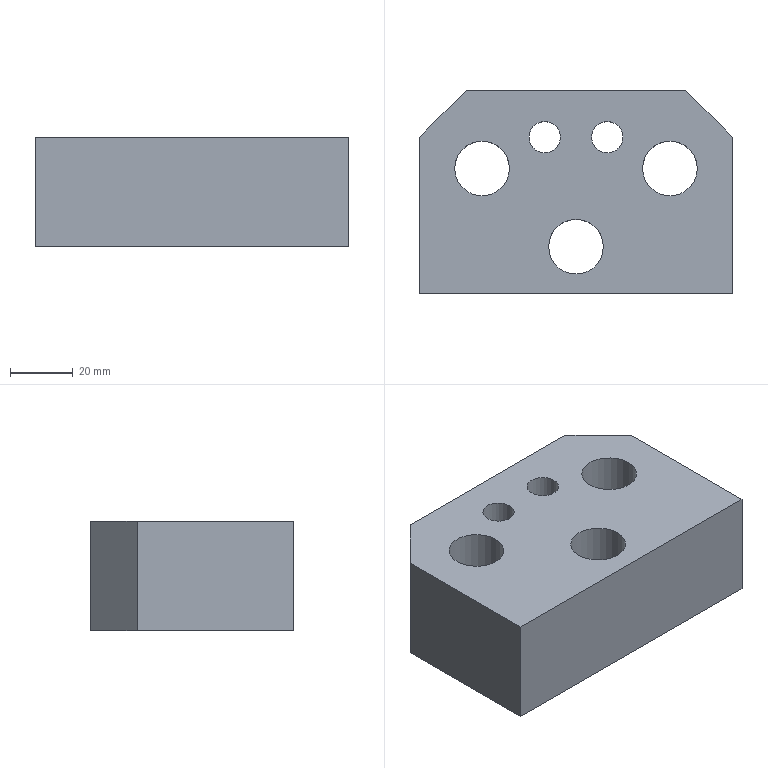Part | NX | features solid 2 | 1 solid | 17 faces | box 100 x 65 x 35 mm | volume 188377 mm3 | plane 10 | cylinder 7 | commonest cylinder face diameters 17.5 x3 10 x2 11 x2
STEP:
#1=CARTESIAN_POINT('',(392.5,-135.,35.));
#2=VERTEX_POINT('',#1);
#3=CARTESIAN_POINT('',(387.5,-135.,35.));
#4=DIRECTION('',(0.,0.,1.));
#5=DIRECTION('',(1.,0.,0.));
#6=AXIS2_PLACEMENT_3D('',#3,#4,#5);
#7=CIRCLE('',#6,5.);
#8=EDGE_CURVE('',#2,#2,#7,.T.);
#9=ORIENTED_EDGE('',*,*,#8,.F.);
#10=EDGE_LOOP('',(#9));
#11=FACE_BOUND('',#10,.T.);
#12=CARTESIAN_POINT('',(412.5,-135.,35.));
#13=VERTEX_POINT('',#12);
#14=CARTESIAN_POINT('',(407.5,-135.,35.));
#15=DIRECTION('',(0.,0.,1.));
#16=DIRECTION('',(1.,0.,0.));
#17=AXIS2_PLACEMENT_3D('',#14,#15,#16);
#18=CIRCLE('',#17,5.);
#19=EDGE_CURVE('',#13,#13,#18,.T.);
#20=ORIENTED_EDGE('',*,*,#19,.F.);
#21=EDGE_LOOP('',(#20));
#22=FACE_BOUND('',#21,.T.);
#23=CARTESIAN_POINT('',(447.5,-185.,35.));
#24=VERTEX_POINT('',#23);
#25=CARTESIAN_POINT('',(347.5,-185.,35.));
#26=VERTEX_POINT('',#25);
#27=CARTESIAN_POINT('',(372.5,-185.,35.));
#28=DIRECTION('',(-1.,0.,0.));
#29=VECTOR('',#28,1000.);
#30=LINE('',#27,#29);
#31=EDGE_CURVE('',#24,#26,#30,.T.);
#32=ORIENTED_EDGE('',*,*,#31,.F.);
#33=CARTESIAN_POINT('',(447.5,-135.,35.));
#34=VERTEX_POINT('',#33);
#35=CARTESIAN_POINT('',(447.5,-190.,35.));
#36=DIRECTION('',(0.,1.,0.));
#37=VECTOR('',#36,1000.);
#38=LINE('',#35,#37);
#39=EDGE_CURVE('',#24,#34,#38,.T.);
#40=ORIENTED_EDGE('',*,*,#39,.T.);
#41=CARTESIAN_POINT('',(432.5,-120.,35.));
#42=VERTEX_POINT('',#41);
#43=CARTESIAN_POINT('',(432.5,-120.,35.));
#44=DIRECTION('',(0.7071,-0.7071,0.));
#45=VECTOR('',#44,1000.);
#46=LINE('',#43,#45);
#47=EDGE_CURVE('',#34,#42,#46,.F.);
#48=ORIENTED_EDGE('',*,*,#47,.T.);
#49=CARTESIAN_POINT('',(362.5,-120.,35.));
#50=VERTEX_POINT('',#49);
#51=CARTESIAN_POINT('',(447.5,-120.,35.));
#52=DIRECTION('',(1.,0.,0.));
#53=VECTOR('',#52,1000.);
#54=LINE('',#51,#53);
#55=EDGE_CURVE('',#50,#42,#54,.T.);
#56=ORIENTED_EDGE('',*,*,#55,.F.);
#57=CARTESIAN_POINT('',(347.5,-135.,35.));
#58=VERTEX_POINT('',#57);
#59=CARTESIAN_POINT('',(337.5,-145.,35.));
#60=DIRECTION('',(0.7071,0.7071,0.));
#61=VECTOR('',#60,1000.);
#62=LINE('',#59,#61);
#63=EDGE_CURVE('',#50,#58,#62,.F.);
#64=ORIENTED_EDGE('',*,*,#63,.T.);
#65=CARTESIAN_POINT('',(347.5,-190.,35.));
#66=DIRECTION('',(0.,1.,0.));
#67=VECTOR('',#66,1000.);
#68=LINE('',#65,#67);
#69=EDGE_CURVE('',#26,#58,#68,.T.);
#70=ORIENTED_EDGE('',*,*,#69,.F.);
#71=EDGE_LOOP('',(#32,#40,#48,#56,#64,#70));
#72=FACE_BOUND('',#71,.T.);
#73=CARTESIAN_POINT('',(376.25,-145.,35.));
#74=VERTEX_POINT('',#73);
#75=CARTESIAN_POINT('',(367.5,-145.,35.));
#76=DIRECTION('',(0.,0.,1.));
#77=DIRECTION('',(1.,0.,0.));
#78=AXIS2_PLACEMENT_3D('',#75,#76,#77);
#79=CIRCLE('',#78,8.75);
#80=EDGE_CURVE('',#74,#74,#79,.T.);
#81=ORIENTED_EDGE('',*,*,#80,.F.);
#82=EDGE_LOOP('',(#81));
#83=FACE_BOUND('',#82,.T.);
#84=CARTESIAN_POINT('',(436.25,-145.,35.));
#85=VERTEX_POINT('',#84);
#86=CARTESIAN_POINT('',(427.5,-145.,35.));
#87=DIRECTION('',(0.,0.,1.));
#88=DIRECTION('',(1.,0.,0.));
#89=AXIS2_PLACEMENT_3D('',#86,#87,#88);
#90=CIRCLE('',#89,8.75);
#91=EDGE_CURVE('',#85,#85,#90,.T.);
#92=ORIENTED_EDGE('',*,*,#91,.F.);
#93=EDGE_LOOP('',(#92));
#94=FACE_BOUND('',#93,.T.);
#95=CARTESIAN_POINT('',(406.25,-170.,35.));
#96=VERTEX_POINT('',#95);
#97=CARTESIAN_POINT('',(397.5,-170.,35.));
#98=DIRECTION('',(0.,0.,1.));
#99=DIRECTION('',(1.,0.,0.));
#100=AXIS2_PLACEMENT_3D('',#97,#98,#99);
#101=CIRCLE('',#100,8.75);
#102=EDGE_CURVE('',#96,#96,#101,.T.);
#103=ORIENTED_EDGE('',*,*,#102,.F.);
#104=EDGE_LOOP('',(#103));
#105=FACE_BOUND('',#104,.T.);
#106=CARTESIAN_POINT('',(372.5,-190.,35.));
#107=DIRECTION('',(0.,0.,1.));
#108=DIRECTION('',(1.,0.,0.));
#109=AXIS2_PLACEMENT_3D('',#106,#107,#108);
#110=PLANE('',#109);
#111=ADVANCED_FACE('',(#11,#22,#72,#83,#94,#105),#110,.T.);
#112=CARTESIAN_POINT('',(447.5,-185.,0.));
#113=VERTEX_POINT('',#112);
#114=CARTESIAN_POINT('',(447.5,-185.,100.));
#115=DIRECTION('',(0.,0.,-1.));
#116=VECTOR('',#115,1000.);
#117=LINE('',#114,#116);
#118=EDGE_CURVE('',#24,#113,#117,.T.);
#119=ORIENTED_EDGE('',*,*,#118,.T.);
#120=CARTESIAN_POINT('',(447.5,-135.,0.));
#121=VERTEX_POINT('',#120);
#122=CARTESIAN_POINT('',(447.5,-190.,0.));
#123=DIRECTION('',(0.,1.,0.));
#124=VECTOR('',#123,1000.);
#125=LINE('',#122,#124);
#126=EDGE_CURVE('',#113,#121,#125,.T.);
#127=ORIENTED_EDGE('',*,*,#126,.T.);
#128=CARTESIAN_POINT('',(447.5,-135.,25.));
#129=DIRECTION('',(0.,0.,1.));
#130=VECTOR('',#129,1000.);
#131=LINE('',#128,#130);
#132=EDGE_CURVE('',#121,#34,#131,.T.);
#133=ORIENTED_EDGE('',*,*,#132,.T.);
#134=ORIENTED_EDGE('',*,*,#39,.F.);
#135=EDGE_LOOP('',(#119,#127,#133,#134));
#136=FACE_BOUND('',#135,.T.);
#137=CARTESIAN_POINT('',(447.5,-190.,25.));
#138=DIRECTION('',(1.,0.,0.));
#139=DIRECTION('',(0.,0.,-1.));
#140=AXIS2_PLACEMENT_3D('',#137,#138,#139);
#141=PLANE('',#140);
#142=ADVANCED_FACE('',(#136),#141,.T.);
#143=CARTESIAN_POINT('',(382.,-135.,0.));
#144=VERTEX_POINT('',#143);
#145=CARTESIAN_POINT('',(387.5,-135.,0.));
#146=DIRECTION('',(0.,0.,-1.));
#147=DIRECTION('',(-1.,0.,0.));
#148=AXIS2_PLACEMENT_3D('',#145,#146,#147);
#149=CIRCLE('',#148,5.5);
#150=EDGE_CURVE('',#144,#144,#149,.T.);
#151=ORIENTED_EDGE('',*,*,#150,.F.);
#152=EDGE_LOOP('',(#151));
#153=FACE_BOUND('',#152,.T.);
#154=CARTESIAN_POINT('',(402.,-135.,0.));
#155=VERTEX_POINT('',#154);
#156=CARTESIAN_POINT('',(407.5,-135.,0.));
#157=DIRECTION('',(0.,0.,-1.));
#158=DIRECTION('',(-1.,0.,0.));
#159=AXIS2_PLACEMENT_3D('',#156,#157,#158);
#160=CIRCLE('',#159,5.5);
#161=EDGE_CURVE('',#155,#155,#160,.T.);
#162=ORIENTED_EDGE('',*,*,#161,.F.);
#163=EDGE_LOOP('',(#162));
#164=FACE_BOUND('',#163,.T.);
#165=CARTESIAN_POINT('',(347.5,-185.,0.));
#166=VERTEX_POINT('',#165);
#167=CARTESIAN_POINT('',(447.5,-185.,0.));
#168=DIRECTION('',(-1.,0.,0.));
#169=VECTOR('',#168,1000.);
#170=LINE('',#167,#169);
#171=EDGE_CURVE('',#113,#166,#170,.T.);
#172=ORIENTED_EDGE('',*,*,#171,.T.);
#173=CARTESIAN_POINT('',(347.5,-135.,0.));
#174=VERTEX_POINT('',#173);
#175=CARTESIAN_POINT('',(347.5,-190.,0.));
#176=DIRECTION('',(0.,1.,0.));
#177=VECTOR('',#176,1000.);
#178=LINE('',#175,#177);
#179=EDGE_CURVE('',#166,#174,#178,.T.);
#180=ORIENTED_EDGE('',*,*,#179,.T.);
#181=CARTESIAN_POINT('',(362.5,-120.,0.));
#182=VERTEX_POINT('',#181);
#183=CARTESIAN_POINT('',(332.5,-150.,0.));
#184=DIRECTION('',(-0.7071,-0.7071,0.));
#185=VECTOR('',#184,1000.);
#186=LINE('',#183,#185);
#187=EDGE_CURVE('',#174,#182,#186,.F.);
#188=ORIENTED_EDGE('',*,*,#187,.T.);
#189=CARTESIAN_POINT('',(432.5,-120.,0.));
#190=VERTEX_POINT('',#189);
#191=CARTESIAN_POINT('',(447.5,-120.,0.));
#192=DIRECTION('',(-1.,0.,0.));
#193=VECTOR('',#192,1000.);
#194=LINE('',#191,#193);
#195=EDGE_CURVE('',#190,#182,#194,.T.);
#196=ORIENTED_EDGE('',*,*,#195,.F.);
#197=CARTESIAN_POINT('',(437.5,-125.,0.));
#198=DIRECTION('',(-0.7071,0.7071,0.));
#199=VECTOR('',#198,1000.);
#200=LINE('',#197,#199);
#201=EDGE_CURVE('',#190,#121,#200,.F.);
#202=ORIENTED_EDGE('',*,*,#201,.T.);
#203=ORIENTED_EDGE('',*,*,#126,.F.);
#204=EDGE_LOOP('',(#172,#180,#188,#196,#202,#203));
#205=FACE_BOUND('',#204,.T.);
#206=CARTESIAN_POINT('',(376.25,-145.,0.));
#207=VERTEX_POINT('',#206);
#208=CARTESIAN_POINT('',(367.5,-145.,0.));
#209=DIRECTION('',(0.,0.,1.));
#210=DIRECTION('',(1.,0.,0.));
#211=AXIS2_PLACEMENT_3D('',#208,#209,#210);
#212=CIRCLE('',#211,8.75);
#213=EDGE_CURVE('',#207,#207,#212,.T.);
#214=ORIENTED_EDGE('',*,*,#213,.T.);
#215=EDGE_LOOP('',(#214));
#216=FACE_BOUND('',#215,.T.);
#217=CARTESIAN_POINT('',(436.25,-145.,0.));
#218=VERTEX_POINT('',#217);
#219=CARTESIAN_POINT('',(427.5,-145.,0.));
#220=DIRECTION('',(0.,0.,1.));
#221=DIRECTION('',(1.,0.,0.));
#222=AXIS2_PLACEMENT_3D('',#219,#220,#221);
#223=CIRCLE('',#222,8.75);
#224=EDGE_CURVE('',#218,#218,#223,.T.);
#225=ORIENTED_EDGE('',*,*,#224,.T.);
#226=EDGE_LOOP('',(#225));
#227=FACE_BOUND('',#226,.T.);
#228=CARTESIAN_POINT('',(406.25,-170.,0.));
#229=VERTEX_POINT('',#228);
#230=CARTESIAN_POINT('',(397.5,-170.,0.));
#231=DIRECTION('',(0.,0.,1.));
#232=DIRECTION('',(1.,0.,0.));
#233=AXIS2_PLACEMENT_3D('',#230,#231,#232);
#234=CIRCLE('',#233,8.75);
#235=EDGE_CURVE('',#229,#229,#234,.T.);
#236=ORIENTED_EDGE('',*,*,#235,.T.);
#237=EDGE_LOOP('',(#236));
#238=FACE_BOUND('',#237,.T.);
#239=CARTESIAN_POINT('',(372.5,-190.,0.));
#240=DIRECTION('',(0.,0.,-1.));
#241=DIRECTION('',(-1.,0.,0.));
#242=AXIS2_PLACEMENT_3D('',#239,#240,#241);
#243=PLANE('',#242);
#244=ADVANCED_FACE('',(#153,#164,#205,#216,#227,#238),#243,.T.);
#245=CARTESIAN_POINT('',(347.5,-185.,0.));
#246=DIRECTION('',(0.,0.,1.));
#247=VECTOR('',#246,1000.);
#248=LINE('',#245,#247);
#249=EDGE_CURVE('',#166,#26,#248,.T.);
#250=ORIENTED_EDGE('',*,*,#249,.T.);
#251=ORIENTED_EDGE('',*,*,#69,.T.);
#252=CARTESIAN_POINT('',(347.5,-135.,-75.));
#253=DIRECTION('',(0.,0.,-1.));
#254=VECTOR('',#253,1000.);
#255=LINE('',#252,#254);
#256=EDGE_CURVE('',#58,#174,#255,.T.);
#257=ORIENTED_EDGE('',*,*,#256,.T.);
#258=ORIENTED_EDGE('',*,*,#179,.F.);
#259=EDGE_LOOP('',(#250,#251,#257,#258));
#260=FACE_BOUND('',#259,.T.);
#261=CARTESIAN_POINT('',(347.5,-190.,-75.));
#262=DIRECTION('',(-1.,0.,0.));
#263=DIRECTION('',(0.,0.,1.));
#264=AXIS2_PLACEMENT_3D('',#261,#262,#263);
#265=PLANE('',#264);
#266=ADVANCED_FACE('',(#260),#265,.T.);
#267=ORIENTED_EDGE('',*,*,#55,.T.);
#268=CARTESIAN_POINT('',(432.5,-120.,25.));
#269=DIRECTION('',(0.,0.,-1.));
#270=VECTOR('',#269,1000.);
#271=LINE('',#268,#270);
#272=EDGE_CURVE('',#42,#190,#271,.T.);
#273=ORIENTED_EDGE('',*,*,#272,.T.);
#274=ORIENTED_EDGE('',*,*,#195,.T.);
#275=CARTESIAN_POINT('',(362.5,-120.,25.));
#276=DIRECTION('',(0.,0.,1.));
#277=VECTOR('',#276,1000.);
#278=LINE('',#275,#277);
#279=EDGE_CURVE('',#182,#50,#278,.T.);
#280=ORIENTED_EDGE('',*,*,#279,.T.);
#281=EDGE_LOOP('',(#267,#273,#274,#280));
#282=FACE_BOUND('',#281,.T.);
#283=CARTESIAN_POINT('',(447.5,-120.,25.));
#284=DIRECTION('',(0.,1.,0.));
#285=DIRECTION('',(-1.,0.,0.));
#286=AXIS2_PLACEMENT_3D('',#283,#284,#285);
#287=PLANE('',#286);
#288=ADVANCED_FACE('',(#282),#287,.T.);
#289=ORIENTED_EDGE('',*,*,#47,.F.);
#290=ORIENTED_EDGE('',*,*,#132,.F.);
#291=ORIENTED_EDGE('',*,*,#201,.F.);
#292=ORIENTED_EDGE('',*,*,#272,.F.);
#293=EDGE_LOOP('',(#289,#290,#291,#292));
#294=FACE_BOUND('',#293,.T.);
#295=CARTESIAN_POINT('',(432.5,-120.,25.));
#296=DIRECTION('',(-0.7071,-0.7071,0.));
#297=DIRECTION('',(0.7071,-0.7071,0.));
#298=AXIS2_PLACEMENT_3D('',#295,#296,#297);
#299=PLANE('',#298);
#300=ADVANCED_FACE('',(#294),#299,.F.);
#301=ORIENTED_EDGE('',*,*,#187,.F.);
#302=ORIENTED_EDGE('',*,*,#256,.F.);
#303=ORIENTED_EDGE('',*,*,#63,.F.);
#304=ORIENTED_EDGE('',*,*,#279,.F.);
#305=EDGE_LOOP('',(#301,#302,#303,#304));
#306=FACE_BOUND('',#305,.T.);
#307=CARTESIAN_POINT('',(362.5,-120.,25.));
#308=DIRECTION('',(0.7071,-0.7071,0.));
#309=DIRECTION('',(0.7071,0.7071,0.));
#310=AXIS2_PLACEMENT_3D('',#307,#308,#309);
#311=PLANE('',#310);
#312=ADVANCED_FACE('',(#306),#311,.F.);
#313=ORIENTED_EDGE('',*,*,#102,.T.);
#314=EDGE_LOOP('',(#313));
#315=FACE_BOUND('',#314,.T.);
#316=ORIENTED_EDGE('',*,*,#235,.F.);
#317=EDGE_LOOP('',(#316));
#318=FACE_BOUND('',#317,.T.);
#319=CARTESIAN_POINT('',(397.5,-170.,125.));
#320=DIRECTION('',(0.,0.,1.));
#321=DIRECTION('',(1.,0.,0.));
#322=AXIS2_PLACEMENT_3D('',#319,#320,#321);
#323=CYLINDRICAL_SURFACE('',#322,8.75);
#324=ADVANCED_FACE('',(#315,#318),#323,.F.);
#325=ORIENTED_EDGE('',*,*,#91,.T.);
#326=EDGE_LOOP('',(#325));
#327=FACE_BOUND('',#326,.T.);
#328=ORIENTED_EDGE('',*,*,#224,.F.);
#329=EDGE_LOOP('',(#328));
#330=FACE_BOUND('',#329,.T.);
#331=CARTESIAN_POINT('',(427.5,-145.,125.));
#332=DIRECTION('',(0.,0.,1.));
#333=DIRECTION('',(1.,0.,0.));
#334=AXIS2_PLACEMENT_3D('',#331,#332,#333);
#335=CYLINDRICAL_SURFACE('',#334,8.75);
#336=ADVANCED_FACE('',(#327,#330),#335,.F.);
#337=ORIENTED_EDGE('',*,*,#80,.T.);
#338=EDGE_LOOP('',(#337));
#339=FACE_BOUND('',#338,.T.);
#340=ORIENTED_EDGE('',*,*,#213,.F.);
#341=EDGE_LOOP('',(#340));
#342=FACE_BOUND('',#341,.T.);
#343=CARTESIAN_POINT('',(367.5,-145.,125.));
#344=DIRECTION('',(0.,0.,1.));
#345=DIRECTION('',(1.,0.,0.));
#346=AXIS2_PLACEMENT_3D('',#343,#344,#345);
#347=CYLINDRICAL_SURFACE('',#346,8.75);
#348=ADVANCED_FACE('',(#339,#342),#347,.F.);
#349=ORIENTED_EDGE('',*,*,#31,.T.);
#350=ORIENTED_EDGE('',*,*,#249,.F.);
#351=ORIENTED_EDGE('',*,*,#171,.F.);
#352=ORIENTED_EDGE('',*,*,#118,.F.);
#353=EDGE_LOOP('',(#349,#350,#351,#352));
#354=FACE_BOUND('',#353,.T.);
#355=CARTESIAN_POINT('',(447.5,-185.,100.));
#356=DIRECTION('',(0.,1.,0.));
#357=DIRECTION('',(-1.,0.,0.));
#358=AXIS2_PLACEMENT_3D('',#355,#356,#357);
#359=PLANE('',#358);
#360=ADVANCED_FACE('',(#354),#359,.F.);
#361=ORIENTED_EDGE('',*,*,#19,.T.);
#362=EDGE_LOOP('',(#361));
#363=FACE_BOUND('',#362,.T.);
#364=CARTESIAN_POINT('',(412.5,-135.,15.));
#365=VERTEX_POINT('',#364);
#366=CARTESIAN_POINT('',(407.5,-135.,15.));
#367=DIRECTION('',(0.,0.,1.));
#368=DIRECTION('',(1.,0.,0.));
#369=AXIS2_PLACEMENT_3D('',#366,#367,#368);
#370=CIRCLE('',#369,5.);
#371=EDGE_CURVE('',#365,#365,#370,.F.);
#372=ORIENTED_EDGE('',*,*,#371,.T.);
#373=EDGE_LOOP('',(#372));
#374=FACE_BOUND('',#373,.T.);
#375=CARTESIAN_POINT('',(407.5,-135.,55.));
#376=DIRECTION('',(0.,0.,-1.));
#377=DIRECTION('',(-1.,0.,0.));
#378=AXIS2_PLACEMENT_3D('',#375,#376,#377);
#379=CYLINDRICAL_SURFACE('',#378,5.);
#380=ADVANCED_FACE('',(#363,#374),#379,.F.);
#381=ORIENTED_EDGE('',*,*,#371,.F.);
#382=EDGE_LOOP('',(#381));
#383=FACE_BOUND('',#382,.T.);
#384=CARTESIAN_POINT('',(402.,-135.,15.));
#385=VERTEX_POINT('',#384);
#386=CARTESIAN_POINT('',(407.5,-135.,15.));
#387=DIRECTION('',(0.,0.,-1.));
#388=DIRECTION('',(-1.,0.,0.));
#389=AXIS2_PLACEMENT_3D('',#386,#387,#388);
#390=CIRCLE('',#389,5.5);
#391=EDGE_CURVE('',#385,#385,#390,.T.);
#392=ORIENTED_EDGE('',*,*,#391,.T.);
#393=EDGE_LOOP('',(#392));
#394=FACE_BOUND('',#393,.T.);
#395=CARTESIAN_POINT('',(404.011,-134.928,15.));
#396=DIRECTION('',(0.,0.,1.));
#397=DIRECTION('',(1.,0.,0.));
#398=AXIS2_PLACEMENT_3D('',#395,#396,#397);
#399=PLANE('',#398);
#400=ADVANCED_FACE('',(#383,#394),#399,.F.);
#401=ORIENTED_EDGE('',*,*,#161,.T.);
#402=EDGE_LOOP('',(#401));
#403=FACE_BOUND('',#402,.T.);
#404=ORIENTED_EDGE('',*,*,#391,.F.);
#405=EDGE_LOOP('',(#404));
#406=FACE_BOUND('',#405,.T.);
#407=CARTESIAN_POINT('',(407.5,-135.,15.));
#408=DIRECTION('',(0.,0.,-1.));
#409=DIRECTION('',(-1.,0.,0.));
#410=AXIS2_PLACEMENT_3D('',#407,#408,#409);
#411=CYLINDRICAL_SURFACE('',#410,5.5);
#412=ADVANCED_FACE('',(#403,#406),#411,.F.);
#413=ORIENTED_EDGE('',*,*,#8,.T.);
#414=EDGE_LOOP('',(#413));
#415=FACE_BOUND('',#414,.T.);
#416=CARTESIAN_POINT('',(392.5,-135.,15.));
#417=VERTEX_POINT('',#416);
#418=CARTESIAN_POINT('',(387.5,-135.,15.));
#419=DIRECTION('',(0.,0.,1.));
#420=DIRECTION('',(1.,0.,0.));
#421=AXIS2_PLACEMENT_3D('',#418,#419,#420);
#422=CIRCLE('',#421,5.);
#423=EDGE_CURVE('',#417,#417,#422,.F.);
#424=ORIENTED_EDGE('',*,*,#423,.T.);
#425=EDGE_LOOP('',(#424));
#426=FACE_BOUND('',#425,.T.);
#427=CARTESIAN_POINT('',(387.5,-135.,55.));
#428=DIRECTION('',(0.,0.,-1.));
#429=DIRECTION('',(-1.,0.,0.));
#430=AXIS2_PLACEMENT_3D('',#427,#428,#429);
#431=CYLINDRICAL_SURFACE('',#430,5.);
#432=ADVANCED_FACE('',(#415,#426),#431,.F.);
#433=ORIENTED_EDGE('',*,*,#423,.F.);
#434=EDGE_LOOP('',(#433));
#435=FACE_BOUND('',#434,.T.);
#436=CARTESIAN_POINT('',(382.,-135.,15.));
#437=VERTEX_POINT('',#436);
#438=CARTESIAN_POINT('',(387.5,-135.,15.));
#439=DIRECTION('',(0.,0.,-1.));
#440=DIRECTION('',(-1.,0.,0.));
#441=AXIS2_PLACEMENT_3D('',#438,#439,#440);
#442=CIRCLE('',#441,5.5);
#443=EDGE_CURVE('',#437,#437,#442,.T.);
#444=ORIENTED_EDGE('',*,*,#443,.T.);
#445=EDGE_LOOP('',(#444));
#446=FACE_BOUND('',#445,.T.);
#447=CARTESIAN_POINT('',(386.757,-134.003,15.));
#448=DIRECTION('',(0.,0.,1.));
#449=DIRECTION('',(1.,0.,0.));
#450=AXIS2_PLACEMENT_3D('',#447,#448,#449);
#451=PLANE('',#450);
#452=ADVANCED_FACE('',(#435,#446),#451,.F.);
#453=ORIENTED_EDGE('',*,*,#150,.T.);
#454=EDGE_LOOP('',(#453));
#455=FACE_BOUND('',#454,.T.);
#456=ORIENTED_EDGE('',*,*,#443,.F.);
#457=EDGE_LOOP('',(#456));
#458=FACE_BOUND('',#457,.T.);
#459=CARTESIAN_POINT('',(387.5,-135.,15.));
#460=DIRECTION('',(0.,0.,-1.));
#461=DIRECTION('',(-1.,0.,0.));
#462=AXIS2_PLACEMENT_3D('',#459,#460,#461);
#463=CYLINDRICAL_SURFACE('',#462,5.5);
#464=ADVANCED_FACE('',(#455,#458),#463,.F.);
#465=CLOSED_SHELL('',(#111,#142,#244,#266,#288,#300,#312,#324,#336,#348,#360,#380,#400,#412,#432,#452,#464));
#466=MANIFOLD_SOLID_BREP('',#465);
#467=(LENGTH_UNIT()NAMED_UNIT(*)SI_UNIT(.MILLI.,.METRE.));
#468=UNCERTAINTY_MEASURE_WITH_UNIT(LENGTH_MEASURE(0.00001),#467,'','');
#469=(NAMED_UNIT(*)PLANE_ANGLE_UNIT()SI_UNIT($,.RADIAN.));
#470=(NAMED_UNIT(*)SI_UNIT($,.STERADIAN.)SOLID_ANGLE_UNIT());
#471=(GEOMETRIC_REPRESENTATION_CONTEXT(3)GLOBAL_UNCERTAINTY_ASSIGNED_CONTEXT((#468))GLOBAL_UNIT_ASSIGNED_CONTEXT((#467,#469,#470))REPRESENTATION_CONTEXT('',''));
#472=ADVANCED_BREP_SHAPE_REPRESENTATION('',(#466),#471);